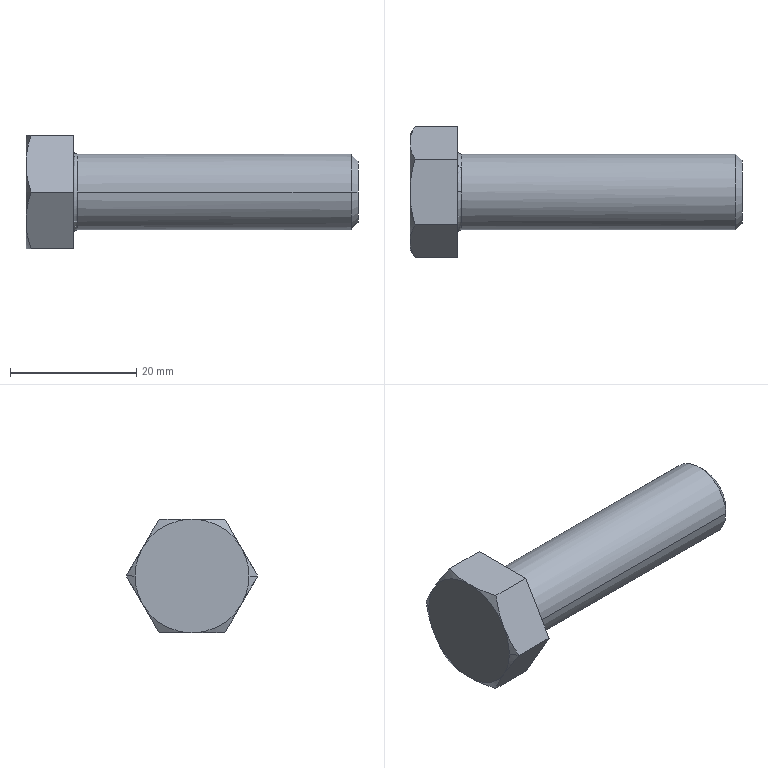Part | STEP file | KS B 1002 - C  M 12 x 45 | 1 solid | 23 faces | box 52.5 x 20.785 x 18 mm | volume 7170 mm3 | cone 10 | plane 9 | torus 2 | cylinder 2 | commonest cylinder face diameters 12 x2